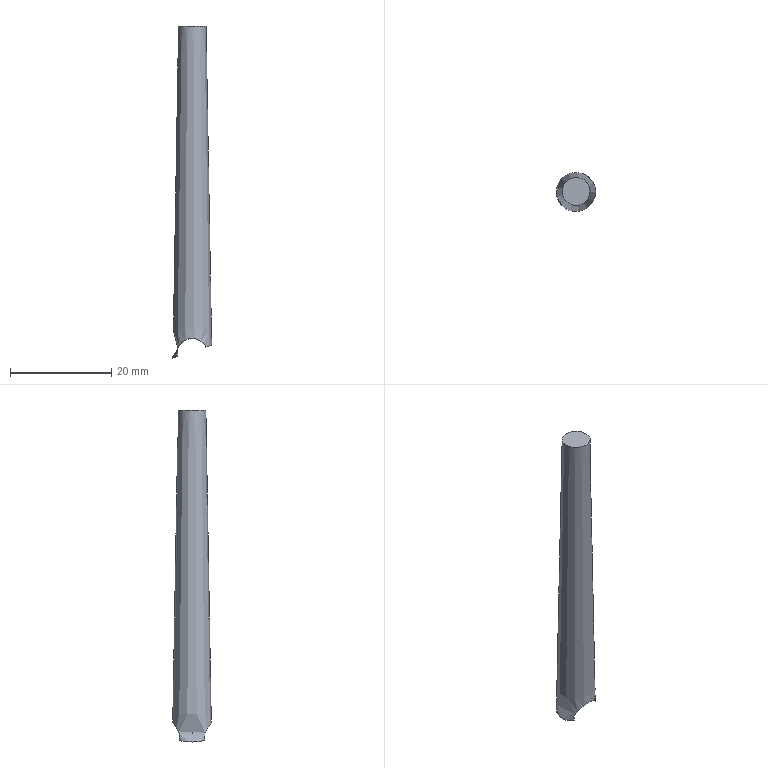Part | NX | features solid 2 | 1 solid | 6 faces | box 7.748 x 7.655 x 65.449 mm | volume 2152 mm3 | cylinder 2 | spline 2 | cone 1 | plane 1 | commonest cylinder face diameters 6 x2
STEP:
#1=CARTESIAN_POINT('',(2.688,0.,16.718));
#2=VERTEX_POINT('',#1);
#3=CARTESIAN_POINT('',(2.724,-2.732,16.729));
#4=VERTEX_POINT('',#3);
#5=CARTESIAN_POINT('',(2.688,0.,16.718));
#6=CARTESIAN_POINT('',(2.7,-0.9106,16.721));
#7=CARTESIAN_POINT('',(2.712,-1.821,16.725));
#8=CARTESIAN_POINT('',(2.724,-2.732,16.729));
#9=B_SPLINE_CURVE_WITH_KNOTS('',3,(#5,#6,#7,#8),.UNSPECIFIED.,.F.,.F.,(4,4),(0.0001813,0.002913),.UNSPECIFIED.);
#10=EDGE_CURVE('',#2,#4,#9,.T.);
#11=ORIENTED_EDGE('',*,*,#10,.T.);
#12=CARTESIAN_POINT('',(-2.934,-2.554,14.89));
#13=VERTEX_POINT('',#12);
#14=CARTESIAN_POINT('',(2.724,-2.732,16.729));
#15=CARTESIAN_POINT('',(2.426,-3.014,17.36));
#16=CARTESIAN_POINT('',(1.683,-3.575,18.129));
#17=CARTESIAN_POINT('',(0.2135,-3.88,18.522));
#18=CARTESIAN_POINT('',(-1.331,-3.729,18.306));
#19=CARTESIAN_POINT('',(-2.446,-3.036,17.373));
#20=CARTESIAN_POINT('',(-2.99,-2.462,16.046));
#21=CARTESIAN_POINT('',(-3.002,-2.467,15.257));
#22=CARTESIAN_POINT('',(-2.934,-2.554,14.89));
#23=B_SPLINE_CURVE_WITH_KNOTS('',3,(#14,#15,#16,#17,#18,#19,#20,#21,#22),.UNSPECIFIED.,.F.,.F.,(4,1,1,1,1,1,4),(0.0004208,0.002678,0.003806,0.004935,0.007191,0.00832,0.009448),.UNSPECIFIED.);
#24=EDGE_CURVE('',#4,#13,#23,.T.);
#25=ORIENTED_EDGE('',*,*,#24,.T.);
#26=CARTESIAN_POINT('',(-2.958,0.,14.882));
#27=VERTEX_POINT('',#26);
#28=CARTESIAN_POINT('',(-2.934,-2.554,14.89));
#29=CARTESIAN_POINT('',(-2.942,-1.703,14.887));
#30=CARTESIAN_POINT('',(-2.95,-0.8514,14.885));
#31=CARTESIAN_POINT('',(-2.958,0.,14.882));
#32=B_SPLINE_CURVE_WITH_KNOTS('',3,(#28,#29,#30,#31),.UNSPECIFIED.,.F.,.F.,(4,4),(0.01171,0.01427),.UNSPECIFIED.);
#33=EDGE_CURVE('',#13,#27,#32,.T.);
#34=ORIENTED_EDGE('',*,*,#33,.T.);
#35=CARTESIAN_POINT('',(-0.0004823,0.,15.387));
#36=DIRECTION('',(0.,1.,0.));
#37=DIRECTION('',(-0.3808,0.,-0.9247));
#38=AXIS2_PLACEMENT_3D('',#35,#36,#37);
#39=ELLIPSE('',#38,3.,3.);
#40=EDGE_CURVE('',#2,#27,#39,.F.);
#41=ORIENTED_EDGE('',*,*,#40,.F.);
#42=EDGE_LOOP('',(#11,#25,#34,#41));
#43=FACE_BOUND('',#42,.T.);
#44=CARTESIAN_POINT('',(0.004771,-0.7587,15.399));
#45=DIRECTION('',(-0.006922,0.9998,-0.01681));
#46=DIRECTION('',(0.,0.01681,0.9999));
#47=AXIS2_PLACEMENT_3D('',#44,#45,#46);
#48=CYLINDRICAL_SURFACE('',#47,3.);
#49=ADVANCED_FACE('',(#43),#48,.F.);
#50=CARTESIAN_POINT('',(-2.934,2.554,14.89));
#51=VERTEX_POINT('',#50);
#52=CARTESIAN_POINT('',(-2.958,0.,14.882));
#53=CARTESIAN_POINT('',(-2.95,0.8514,14.885));
#54=CARTESIAN_POINT('',(-2.942,1.703,14.887));
#55=CARTESIAN_POINT('',(-2.934,2.554,14.89));
#56=B_SPLINE_CURVE_WITH_KNOTS('',3,(#52,#53,#54,#55),.UNSPECIFIED.,.F.,.F.,(4,4),(0.0001113,0.002666),.UNSPECIFIED.);
#57=EDGE_CURVE('',#27,#51,#56,.T.);
#58=ORIENTED_EDGE('',*,*,#57,.T.);
#59=CARTESIAN_POINT('',(2.724,2.732,16.729));
#60=VERTEX_POINT('',#59);
#61=CARTESIAN_POINT('',(-2.934,2.554,14.89));
#62=CARTESIAN_POINT('',(-3.002,2.467,15.256));
#63=CARTESIAN_POINT('',(-2.991,2.461,16.041));
#64=CARTESIAN_POINT('',(-2.449,3.034,17.371));
#65=CARTESIAN_POINT('',(-1.337,3.725,18.301));
#66=CARTESIAN_POINT('',(0.2022,3.88,18.523));
#67=CARTESIAN_POINT('',(1.679,3.578,18.132));
#68=CARTESIAN_POINT('',(2.423,3.016,17.366));
#69=CARTESIAN_POINT('',(2.724,2.732,16.729));
#70=B_SPLINE_CURVE_WITH_KNOTS('',3,(#61,#62,#63,#64,#65,#66,#67,#68,#69),.UNSPECIFIED.,.F.,.F.,(4,1,1,1,1,1,4),(0.000008928,0.00114,0.002271,0.004533,0.005664,0.006795,0.009057),.UNSPECIFIED.);
#71=EDGE_CURVE('',#51,#60,#70,.T.);
#72=ORIENTED_EDGE('',*,*,#71,.T.);
#73=CARTESIAN_POINT('',(2.724,2.732,16.729));
#74=CARTESIAN_POINT('',(2.712,1.821,16.725));
#75=CARTESIAN_POINT('',(2.7,0.9106,16.721));
#76=CARTESIAN_POINT('',(2.688,0.,16.718));
#77=B_SPLINE_CURVE_WITH_KNOTS('',3,(#73,#74,#75,#76),.UNSPECIFIED.,.F.,.F.,(4,4),(0.01146,0.0142),.UNSPECIFIED.);
#78=EDGE_CURVE('',#60,#2,#77,.T.);
#79=ORIENTED_EDGE('',*,*,#78,.T.);
#80=ORIENTED_EDGE('',*,*,#40,.T.);
#81=EDGE_LOOP('',(#58,#72,#79,#80));
#82=FACE_BOUND('',#81,.T.);
#83=CARTESIAN_POINT('',(0.004771,0.7587,15.399));
#84=DIRECTION('',(-0.006922,-0.9998,-0.01681));
#85=DIRECTION('',(0.,-0.01681,0.9999));
#86=AXIS2_PLACEMENT_3D('',#83,#84,#85);
#87=CYLINDRICAL_SURFACE('',#86,3.);
#88=ADVANCED_FACE('',(#82),#87,.F.);
#89=ORIENTED_EDGE('',*,*,#78,.F.);
#90=CARTESIAN_POINT('',(2.724,2.732,16.729));
#91=CARTESIAN_POINT('',(3.43,2.023,16.943));
#92=CARTESIAN_POINT('',(4.277,0.001442,17.19));
#93=CARTESIAN_POINT('',(3.425,-2.028,16.941));
#94=CARTESIAN_POINT('',(2.724,-2.732,16.729));
#95=B_SPLINE_CURVE_WITH_KNOTS('',3,(#90,#91,#92,#93,#94),.UNSPECIFIED.,.F.,.F.,(4,1,4),(0.006855,0.009895,0.01294),.UNSPECIFIED.);
#96=EDGE_CURVE('',#60,#4,#95,.T.);
#97=ORIENTED_EDGE('',*,*,#96,.T.);
#98=ORIENTED_EDGE('',*,*,#10,.F.);
#99=EDGE_LOOP('',(#89,#97,#98));
#100=FACE_BOUND('',#99,.T.);
#101=CARTESIAN_POINT('',(2.681,2.765,16.716));
#102=CARTESIAN_POINT('',(2.681,-2.765,16.716));
#103=CARTESIAN_POINT('',(3.08,2.765,16.837));
#104=CARTESIAN_POINT('',(3.08,-2.765,16.837));
#105=CARTESIAN_POINT('',(3.479,2.765,16.956));
#106=CARTESIAN_POINT('',(3.479,-2.765,16.956));
#107=CARTESIAN_POINT('',(3.878,2.765,17.074));
#108=CARTESIAN_POINT('',(3.878,-2.765,17.074));
#109=B_SPLINE_SURFACE_WITH_KNOTS('',3,1,((#101,#102),(#103,#104),(#105,#106),(#107,#108)),.SURF_OF_LINEAR_EXTRUSION.,.F.,.F.,.F.,(4,4),(2,2),(0.7101,0.7171),(0.,1.),.PIECEWISE_BEZIER_KNOTS.);
#110=ADVANCED_FACE('',(#100),#109,.T.);
#111=ORIENTED_EDGE('',*,*,#33,.F.);
#112=CARTESIAN_POINT('',(-2.934,-2.554,14.89));
#113=CARTESIAN_POINT('',(-3.534,-1.871,14.682));
#114=CARTESIAN_POINT('',(-4.257,-0.007897,14.422));
#115=CARTESIAN_POINT('',(-3.537,1.868,14.68));
#116=CARTESIAN_POINT('',(-2.934,2.554,14.89));
#117=B_SPLINE_CURVE_WITH_KNOTS('',3,(#112,#113,#114,#115,#116),.UNSPECIFIED.,.F.,.F.,(4,1,4),(0.01951,0.02231,0.02511),.UNSPECIFIED.);
#118=EDGE_CURVE('',#13,#51,#117,.T.);
#119=ORIENTED_EDGE('',*,*,#118,.T.);
#120=ORIENTED_EDGE('',*,*,#57,.F.);
#121=EDGE_LOOP('',(#111,#119,#120));
#122=FACE_BOUND('',#121,.T.);
#123=CARTESIAN_POINT('',(-3.919,2.585,14.543));
#124=CARTESIAN_POINT('',(-3.919,-2.585,14.543));
#125=CARTESIAN_POINT('',(-3.589,2.585,14.661));
#126=CARTESIAN_POINT('',(-3.589,-2.585,14.661));
#127=CARTESIAN_POINT('',(-3.259,2.585,14.777));
#128=CARTESIAN_POINT('',(-3.259,-2.585,14.777));
#129=CARTESIAN_POINT('',(-2.928,2.585,14.892));
#130=CARTESIAN_POINT('',(-2.928,-2.585,14.892));
#131=B_SPLINE_SURFACE_WITH_KNOTS('',3,1,((#123,#124),(#125,#126),(#127,#128),(#129,#130)),.SURF_OF_LINEAR_EXTRUSION.,.F.,.F.,.F.,(4,4),(2,2),(0.671,0.6769),(0.,1.),.PIECEWISE_BEZIER_KNOTS.);
#132=ADVANCED_FACE('',(#122),#131,.T.);
#133=CARTESIAN_POINT('',(2.754,0.,80.));
#134=VERTEX_POINT('',#133);
#135=CARTESIAN_POINT('',(0.,0.,80.));
#136=DIRECTION('',(0.,0.,1.));
#137=DIRECTION('',(1.,0.,0.));
#138=AXIS2_PLACEMENT_3D('',#135,#136,#137);
#139=CIRCLE('',#138,2.754);
#140=EDGE_CURVE('',#134,#134,#139,.T.);
#141=ORIENTED_EDGE('',*,*,#140,.F.);
#142=EDGE_LOOP('',(#141));
#143=FACE_BOUND('',#142,.T.);
#144=ORIENTED_EDGE('',*,*,#118,.F.);
#145=ORIENTED_EDGE('',*,*,#24,.F.);
#146=ORIENTED_EDGE('',*,*,#96,.F.);
#147=ORIENTED_EDGE('',*,*,#71,.F.);
#148=EDGE_LOOP('',(#144,#145,#146,#147));
#149=FACE_BOUND('',#148,.T.);
#150=CARTESIAN_POINT('',(0.,0.,137.5));
#151=DIRECTION('',(0.,0.,-1.));
#152=DIRECTION('',(1.,0.,0.));
#153=AXIS2_PLACEMENT_3D('',#150,#151,#152);
#154=CONICAL_SURFACE('',#153,1.75,0.01745);
#155=ADVANCED_FACE('',(#143,#149),#154,.T.);
#156=ORIENTED_EDGE('',*,*,#140,.T.);
#157=EDGE_LOOP('',(#156));
#158=FACE_BOUND('',#157,.T.);
#159=CARTESIAN_POINT('',(0.,0.,80.));
#160=DIRECTION('',(0.,0.,1.));
#161=DIRECTION('',(-1.,0.,0.));
#162=AXIS2_PLACEMENT_3D('',#159,#160,#161);
#163=PLANE('',#162);
#164=ADVANCED_FACE('',(#158),#163,.T.);
#165=CLOSED_SHELL('',(#49,#88,#110,#132,#155,#164));
#166=MANIFOLD_SOLID_BREP('',#165);
#167=(LENGTH_UNIT()NAMED_UNIT(*)SI_UNIT(.MILLI.,.METRE.));
#168=UNCERTAINTY_MEASURE_WITH_UNIT(LENGTH_MEASURE(0.0508),#167,'','');
#169=(NAMED_UNIT(*)PLANE_ANGLE_UNIT()SI_UNIT($,.RADIAN.));
#170=(NAMED_UNIT(*)SI_UNIT($,.STERADIAN.)SOLID_ANGLE_UNIT());
#171=(GEOMETRIC_REPRESENTATION_CONTEXT(3)GLOBAL_UNCERTAINTY_ASSIGNED_CONTEXT((#168))GLOBAL_UNIT_ASSIGNED_CONTEXT((#167,#169,#170))REPRESENTATION_CONTEXT('',''));
#172=ADVANCED_BREP_SHAPE_REPRESENTATION('',(#166),#171);